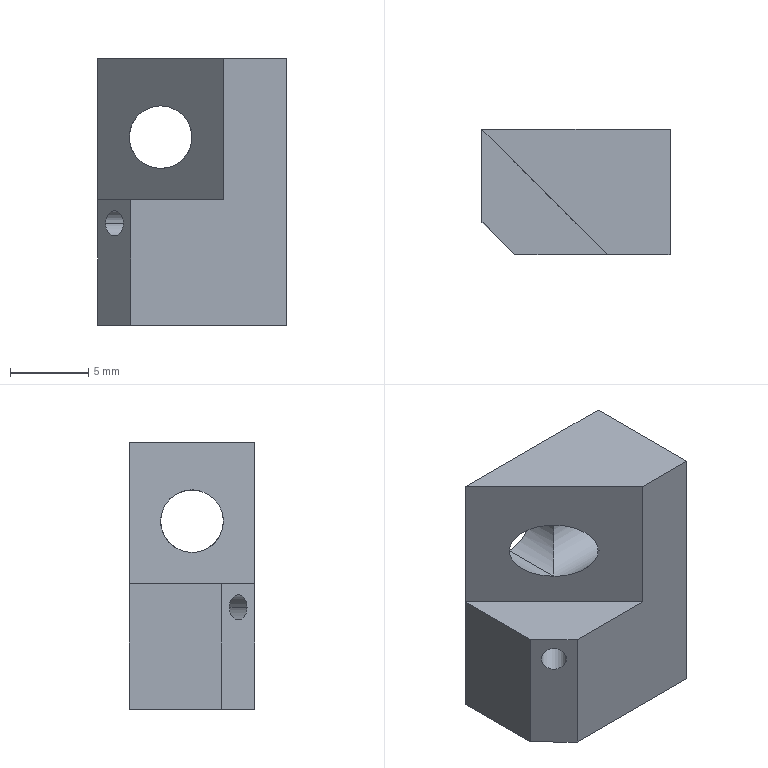NC program | NX | posted with a generic post | part box 12 x 8 x 17 mm
Whole program:
N10 G17 G21 G94 G90
(FLOOR_WALL , TOOL : D10JING)
N12 T09 M6
N14 G54
N16 G17 G0 G90 X-16. Y4.997 S9500 M3
N18 G43 Z30. H9
N20 Z3.
N22 G94 G1 Z0. F1250.
N24 X-13.
N26 X13.
N28 Y1.999
N30 X-13.
N32 Y-1.
N34 X13.
N36 X16.
N38 Z3.
N40 G0 Z30.
N42 M5
(FLOOR_WALL_1 , TOOL : D6)
N44 T06 M6
N46 G54
N48 G17 G0 G90 X-0.777 Y-9. S9500 M3
N50 G43 Z30. H6
N52 Z-0.297
N54 G94 G1 X-1.759 Y-7.3 F1000.
N56 G3 X-2.278 Y-7. R0.6
N58 G1 X-5.143 F2500.
N60 X-9. Y-3.143
N62 Y2.586
N64 X-8.97
N66 X0.586 Y-6.97
N68 Y-7.
N70 X-2.278
N72 G3 X-2.798 Y-7.3 R0.6
N74 G1 X-3.779 Y-9.
N76 G0 X-0.777 Z-0.593
N78 G1 X-1.759 Y-7.3 F1000.
N80 G3 X-2.278 Y-7. R0.6
N82 G1 X-5.143 F2500.
N84 X-9. Y-3.143
N86 Y2.586
N88 X-8.97
N90 X0.586 Y-6.97
N92 Y-7.
N94 X-2.278
N96 G3 X-2.798 Y-7.3 R0.6
N98 G1 X-3.779 Y-9.
N100 G0 X-0.777 Z-0.89
N102 G1 X-1.759 Y-7.3 F1000.
N104 G3 X-2.278 Y-7. R0.6
N106 G1 X-5.143 F2500.
N108 X-9. Y-3.143
N110 Y2.586
N112 X-8.97
N114 X0.586 Y-6.97
N116 Y-7.
N118 X-2.278
N120 G3 X-2.798 Y-7.3 R0.6
N122 G1 X-3.779 Y-9.
N124 G0 X-0.777 Z-1.187
N126 G1 X-1.759 Y-7.3 F1000.
N128 G3 X-2.278 Y-7. R0.6
N130 G1 X-5.143 F2500.
N132 X-9. Y-3.143
N134 Y2.586
N136 X-8.97
N138 X0.586 Y-6.97
N140 Y-7.
N142 X-2.278
N144 G3 X-2.798 Y-7.3 R0.6
N146 G1 X-3.779 Y-9.
N148 G0 X-0.777 Z-1.483
N150 G1 X-1.759 Y-7.3 F1000.
N152 G3 X-2.278 Y-7. R0.6
N154 G1 X-5.143 F2500.
N156 X-9. Y-3.143
N158 Y2.586
N160 X-8.97
N162 X0.586 Y-6.97
N164 Y-7.
N166 X-2.278
N168 G3 X-2.798 Y-7.3 R0.6
N170 G1 X-3.779 Y-9.
N172 G0 X-0.777 Z-1.78
N174 G1 X-1.759 Y-7.3 F1000.
N176 G3 X-2.278 Y-7. R0.6
N178 G1 X-5.143 F2500.
N180 X-9. Y-3.143
N182 Y2.586
N184 X-8.97
N186 X0.586 Y-6.97
N188 Y-7.
N190 X-2.278
N192 G3 X-2.798 Y-7.3 R0.6
N194 G1 X-3.779 Y-9.
N196 G0 X-0.777 Z-2.077
N198 G1 X-1.759 Y-7.3 F1000.
N200 G3 X-2.278 Y-7. R0.6
N202 G1 X-5.143 F2500.
N204 X-9. Y-3.143
N206 Y2.586
N208 X-8.97
N210 X0.586 Y-6.97
N212 Y-7.
N214 X-2.278
N216 G3 X-2.798 Y-7.3 R0.6
N218 G1 X-3.779 Y-9.
N220 G0 X-0.777 Z-2.373
N222 G1 X-1.759 Y-7.3 F1000.
N224 G3 X-2.278 Y-7. R0.6
N226 G1 X-5.143 F2500.
N228 X-9. Y-3.143
N230 Y2.586
N232 X-8.97
N234 X0.586 Y-6.97
N236 Y-7.
N238 X-2.278
N240 G3 X-2.798 Y-7.3 R0.6
N242 G1 X-3.779 Y-9.
N244 G0 X-0.777 Z-2.67
N246 G1 X-1.759 Y-7.3 F1000.
N248 G3 X-2.278 Y-7. R0.6
N250 G1 X-5.143 F2500.
N252 X-9. Y-3.143
N254 Y2.586
N256 X-8.97
N258 X0.586 Y-6.97
N260 Y-7.
N262 X-2.278
N264 G3 X-2.798 Y-7.3 R0.6
N266 G1 X-3.779 Y-9.
N268 G0 X-0.777 Z-2.967
N270 G1 X-1.759 Y-7.3 F1000.
N272 G3 X-2.278 Y-7. R0.6
N274 G1 X-5.143 F2500.
N276 X-9. Y-3.143
N278 Y2.586
N280 X-8.97
N282 X0.586 Y-6.97
N284 Y-7.
N286 X-2.278
N288 G3 X-2.798 Y-7.3 R0.6
N290 G1 X-3.779 Y-9.
N292 G0 X-0.777 Z-3.263
N294 G1 X-1.759 Y-7.3 F1000.
N296 G3 X-2.278 Y-7. R0.6
N298 G1 X-5.143 F2500.
N300 X-9. Y-3.143
N302 Y2.586
N304 X-8.97
N306 X0.586 Y-6.97
N308 Y-7.
N310 X-2.278
N312 G3 X-2.798 Y-7.3 R0.6
N314 G1 X-3.779 Y-9.
N316 G0 X-0.777 Z-3.56
N318 G1 X-1.759 Y-7.3 F1000.
N320 G3 X-2.278 Y-7. R0.6
N322 G1 X-5.143 F2500.
N324 X-9. Y-3.143
N326 Y2.586
N328 X-8.97
N330 X0.586 Y-6.97
N332 Y-7.
N334 X-2.278
N336 G3 X-2.798 Y-7.3 R0.6
N338 G1 X-3.779 Y-9.
N340 G0 X-0.777 Z-3.857
N342 G1 X-1.759 Y-7.3 F1000.
N344 G3 X-2.278 Y-7. R0.6
N346 G1 X-5.143 F2500.
N348 X-9. Y-3.143
N350 Y2.586
N352 X-8.97
N354 X0.586 Y-6.97
N356 Y-7.
N358 X-2.278
N360 G3 X-2.798 Y-7.3 R0.6
N362 G1 X-3.779 Y-9.
N364 G0 X-0.777 Z-4.153
N366 G1 X-1.759 Y-7.3 F1000.
N368 G3 X-2.278 Y-7. R0.6
N370 G1 X-5.143 F2500.
N372 X-9. Y-3.143
N374 Y2.586
N376 X-8.97
N378 X0.586 Y-6.97
N380 Y-7.
N382 X-2.278
N384 G3 X-2.798 Y-7.3 R0.6
N386 G1 X-3.779 Y-9.
N388 G0 X-0.777 Z-4.45
N390 G1 X-1.759 Y-7.3 F1000.
N392 G3 X-2.278 Y-7. R0.6
N394 G1 X-5.143 F2500.
N396 X-9. Y-3.143
N398 Y2.586
N400 X-8.97
N402 X0.586 Y-6.97
N404 Y-7.
N406 X-2.278
N408 G3 X-2.798 Y-7.3 R0.6
N410 G1 X-3.779 Y-9.
N412 G0 X-0.777 Z-4.747
N414 G1 X-1.759 Y-7.3 F1000.
N416 G3 X-2.278 Y-7. R0.6
N418 G1 X-5.143 F2500.
N420 X-9. Y-3.143
N422 Y2.586
N424 X-8.97
N426 X0.586 Y-6.97
N428 Y-7.
N430 X-2.278
N432 G3 X-2.798 Y-7.3 R0.6
N434 G1 X-3.779 Y-9.
N436 G0 X-0.777 Z-5.043
N438 G1 X-1.759 Y-7.3 F1000.
N440 G3 X-2.278 Y-7. R0.6
N442 G1 X-5.143 F2500.
N444 X-9. Y-3.143
N446 Y2.586
N448 X-8.97
N450 X0.586 Y-6.97
N452 Y-7.
N454 X-2.278
N456 G3 X-2.798 Y-7.3 R0.6
N458 G1 X-3.779 Y-9.
N460 G0 X-0.777 Z-5.34
N462 G1 X-1.759 Y-7.3 F1000.
N464 G3 X-2.278 Y-7. R0.6
N466 G1 X-5.143 F2500.
N468 X-9. Y-3.143
N470 Y2.586
N472 X-8.97
N474 X0.586 Y-6.97
N476 Y-7.
N478 X-2.278
N480 G3 X-2.798 Y-7.3 R0.6
N482 G1 X-3.779 Y-9.
N484 G0 X-0.777 Z-5.637
N486 G1 X-1.759 Y-7.3 F1000.
N488 G3 X-2.278 Y-7. R0.6
N490 G1 X-5.143 F2500.
N492 X-9. Y-3.143
N494 Y2.586
N496 X-8.97
N498 X0.586 Y-6.97
N500 Y-7.
N502 X-2.278
N504 G3 X-2.798 Y-7.3 R0.6
N506 G1 X-3.779 Y-9.
N508 G0 X-0.777 Z-5.933
N510 G1 X-1.759 Y-7.3 F1000.
N512 G3 X-2.278 Y-7. R0.6
N514 G1 X-5.143 F2500.
N516 X-9. Y-3.143
N518 Y2.586
N520 X-8.97
N522 X0.586 Y-6.97
N524 Y-7.
N526 X-2.278
N528 G3 X-2.798 Y-7.3 R0.6
N530 G1 X-3.779 Y-9.
N532 G0 X-0.777 Z-6.23
N534 G1 X-1.759 Y-7.3 F1000.
N536 G3 X-2.278 Y-7. R0.6
N538 G1 X-5.143 F2500.
N540 X-9. Y-3.143
N542 Y2.586
N544 X-8.97
N546 X0.586 Y-6.97
N548 Y-7.
N550 X-2.278
N552 G3 X-2.798 Y-7.3 R0.6
N554 G1 X-3.779 Y-9.
N556 G0 X-0.777 Z-6.527
N558 G1 X-1.759 Y-7.3 F1000.
N560 G3 X-2.278 Y-7. R0.6
N562 G1 X-5.143 F2500.
N564 X-9. Y-3.143
N566 Y2.586
N568 X-8.97
N570 X0.586 Y-6.97
N572 Y-7.
N574 X-2.278
N576 G3 X-2.798 Y-7.3 R0.6
N578 G1 X-3.779 Y-9.
N580 G0 X-0.777 Z-6.823
N582 G1 X-1.759 Y-7.3 F1000.
N584 G3 X-2.278 Y-7. R0.6
N586 G1 X-5.143 F2500.
N588 X-9. Y-3.143
N590 Y2.586
N592 X-8.97
N594 X0.586 Y-6.97
N596 Y-7.
N598 X-2.278
N600 G3 X-2.798 Y-7.3 R0.6
N602 G1 X-3.779 Y-9.
N604 G0 X-0.777 Z-7.12
N606 G1 X-1.759 Y-7.3 F1000.
N608 G3 X-2.278 Y-7. R0.6
N610 G1 X-5.143 F2500.
N612 X-9. Y-3.143
N614 Y2.586
N616 X-8.97
N618 X0.586 Y-6.97
N620 Y-7.
N622 X-2.278
N624 G3 X-2.798 Y-7.3 R0.6
N626 G1 X-3.779 Y-9.
N628 G0 X-0.777 Z-7.417
N630 G1 X-1.759 Y-7.3 F1000.
N632 G3 X-2.278 Y-7. R0.6
N634 G1 X-5.143 F2500.
N636 X-9. Y-3.143
N638 Y2.586
N640 X-8.97
N642 X0.586 Y-6.97
N644 Y-7.
N646 X-2.278
N648 G3 X-2.798 Y-7.3 R0.6
N650 G1 X-3.779 Y-9.
N652 G0 X-0.777 Z-7.713
N654 G1 X-1.759 Y-7.3 F1000.
N656 G3 X-2.278 Y-7. R0.6
N658 G1 X-5.143 F2500.
N660 X-9. Y-3.143
N662 Y2.586
N664 X-8.97
N666 X0.586 Y-6.97
N668 Y-7.
N670 X-2.278
N672 G3 X-2.798 Y-7.3 R0.6
N674 G1 X-3.779 Y-9.
N676 G0 X-0.777 Z-8.01
N678 G1 X-1.759 Y-7.3 F1000.
N680 G3 X-2.278 Y-7. R0.6
N682 G1 X-5.143 F2500.
N684 X-9. Y-3.143
N686 Y2.586
N688 X-8.97
N690 X0.586 Y-6.97
N692 Y-7.
N694 X-2.278
N696 G3 X-2.798 Y-7.3 R0.6
N698 G1 X-3.779 Y-9.
N700 G0 X-0.777 Z-8.307
N702 G1 X-1.759 Y-7.3 F1000.
N704 G3 X-2.278 Y-7. R0.6
N706 G1 X-5.143 F2500.
N708 X-9. Y-3.143
N710 Y2.586
N712 X-8.97
N714 X0.586 Y-6.97
N716 Y-7.
N718 X-2.278
N720 G3 X-2.798 Y-7.3 R0.6
N722 G1 X-3.779 Y-9.
N724 G0 X-0.777 Z-8.603
N726 G1 X-1.759 Y-7.3 F1000.
N728 G3 X-2.278 Y-7. R0.6
N730 G1 X-5.143 F2500.
N732 X-9. Y-3.143
N734 Y2.586
N736 X-8.97
N738 X0.586 Y-6.97
N740 Y-7.
N742 X-2.278
N744 G3 X-2.798 Y-7.3 R0.6
N746 G1 X-3.779 Y-9.
N748 G0 X-0.777 Z-8.9
N750 G1 X-1.759 Y-7.3 F1000.
N752 G3 X-2.278 Y-7. R0.6
N754 G1 X-5.143 F2500.
N756 X-9. Y-3.143
N758 Y2.586
N760 X-8.97
N762 X0.586 Y-6.97
N764 Y-7.
N766 X-2.278
N768 G3 X-2.798 Y-7.3 R0.6
N770 G1 X-3.779 Y-9.
N772 G0 Z30.
(FLOOR_WALL_1_COPY , TOOL : D6)
N774 X-0.904
N776 Z-9.
N778 G1 X-1.885 Y-7.3 F1000.
N780 G3 X-2.405 Y-7. R0.6
N782 G1 X-5.143 F1200.
N784 X-9. Y-3.143
N786 Y2.333
N788 X0.333 Y-7.
N790 X-2.405
N792 G3 X-2.924 Y-7.3 R0.6
N794 G1 X-3.906 Y-9.
N796 X0.532
N798 X0.913 Y-7.58 F1000.
N800 G3 X0.757 Y-7. R0.6
N802 G1 X-9. Y2.757 F1200.
N804 G3 X-9.58 Y2.913 R0.6
N806 G1 X-11.476 Y2.405
N808 G0 Z30.
N810 M5
(ZLEVEL_PROFILE_1_COPY , TOOL : D6A45)
N812 T07 M6
N814 G54
N816 G17 G0 G90 X-6.923 Y5.953 S9500 M3
N818 G43 Z30. H7
N820 Z1.
N822 G94 G1 Z-1. F1250.
N824 X-6.522 Y5.259
N826 G3 X-6.003 Y4.959 R0.6
N828 G1 X6.003
N830 G2 X6.959 Y4.003 R0.956
N832 G1 Y-4.003
N834 G2 X6.003 Y-4.959 R0.956
N836 G1 X1.997
N838 G2 X1.324 Y-4.68 R0.952
N840 G1 X-6.68 Y3.324
N842 G2 X-6.003 Y4.959 R0.957
N844 G3 X-5.483 Y5.259 R0.6
N846 G1 X-4.963 Y6.159
N848 Z1.
N850 G0 Z30.
N852 M5
(ZLEVEL_PROFILE_COPY_COPY_COPY_COPY_COPY , TOOL : D6)
N854 T06 M6
N856 G54
N858 G17 G0 G90 X-6.973 Y8.086 S9500 M3
N860 G43 Z30. H6
N862 Z-8.5
N864 G94 G1 Z-10. F1000.
N866 X-6.52 Y7.3
N868 G3 X-6. Y7. R0.6
N870 G1 X6. F1200.
N872 G2 X9. Y4. R3.
N874 G1 Y-4.
N876 G2 X6. Y-7. R3.
N878 G1 X-3.9
N880 G2 X-6.021 Y-6.121 R3.
N882 G1 X-8.121 Y-4.021
N884 G2 X-9. Y-1.9 R3.
N886 G1 Y4.
N888 G2 X-6. Y7. R3.
N890 G1 X5.754 Z-11.863
N892 X5.927 Z-11.891
N894 X6.1 Y6.998 Z-11.918
N896 X6.273 Y6.988 Z-11.945
N898 X6.444 Y6.967 Z-11.973
N900 X6.614 Y6.936 Z-12.
N902 X6.782 Y6.896 Z-12.028
N904 X6.948 Y6.846 Z-12.055
N906 X7.11 Y6.787 Z-12.082
N908 X7.269 Y6.718 Z-12.11
N910 X7.423 Y6.641 Z-12.137
N912 X7.573 Y6.555 Z-12.165
N914 X7.718 Y6.46 Z-12.192
N916 X7.856 Y6.357 Z-12.219
N918 X7.989 Y6.246 Z-12.247
N920 X8.115 Y6.128 Z-12.274
N922 X8.234 Y6.002 Z-12.302
N924 X8.346 Y5.87 Z-12.329
N926 X8.449 Y5.732 Z-12.356
N928 X8.545 Y5.588 Z-12.384
N930 X8.632 Y5.439 Z-12.411
N932 X8.711 Y5.285 Z-12.439
N934 X8.78 Y5.127 Z-12.466
N936 X8.841 Y4.965 Z-12.493
N938 X8.891 Y4.8 Z-12.521
N940 X8.933 Y4.632 Z-12.548
N942 X8.964 Y4.462 Z-12.576
N944 X8.986 Y4.29 Z-12.603
N946 X8.998 Y4.118 Z-12.63
N948 X9. Y3.945 Z-12.658
N950 Y3.772 Z-12.685
N952 Y-3.833 Z-13.891
N954 Y-4.006 Z-13.918
N956 X8.995 Y-4.179 Z-13.946
N958 X8.979 Y-4.351 Z-13.973
N960 X8.954 Y-4.522 Z-14.
N962 X8.919 Y-4.691 Z-14.028
N964 X8.875 Y-4.858 Z-14.055
N966 X8.82 Y-5.023 Z-14.083
N968 X8.757 Y-5.183 Z-14.11
N970 X8.684 Y-5.34 Z-14.137
N972 X8.602 Y-5.492 Z-14.165
N974 X8.512 Y-5.64 Z-14.192
N976 X8.414 Y-5.782 Z-14.22
N978 X8.307 Y-5.918 Z-14.247
N980 X8.193 Y-6.047 Z-14.274
N982 X8.071 Y-6.17 Z-14.302
N984 X7.943 Y-6.286 Z-14.329
N986 X7.808 Y-6.394 Z-14.357
N988 X7.667 Y-6.494 Z-14.384
N990 X7.521 Y-6.586 Z-14.411
N992 X7.369 Y-6.669 Z-14.439
N994 X7.213 Y-6.744 Z-14.466
N996 X7.053 Y-6.809 Z-14.494
N998 X6.89 Y-6.865 Z-14.521
N1000 X6.723 Y-6.912 Z-14.548
N1002 X6.554 Y-6.948 Z-14.576
N1004 X6.384 Y-6.975 Z-14.603
N1006 X6.212 Y-6.993 Z-14.631
N1008 X6.039 Y-7. Z-14.658
N1010 X5.866 Z-14.685
N1012 X5.693 Z-14.713
N1014 X-3.641 Z-16.192
N1016 X-3.814 Z-16.22
N1018 X-3.987 Y-6.999 Z-16.247
N1020 X-4.159 Y-6.989 Z-16.275
N1022 X-4.331 Y-6.969 Z-16.302
N1024 X-4.501 Y-6.939 Z-16.329
N1026 X-4.67 Y-6.9 Z-16.357
N1028 X-4.835 Y-6.85 Z-16.384
N1030 X-4.998 Y-6.792 Z-16.412
N1032 X-5.157 Y-6.724 Z-16.439
N1034 X-5.312 Y-6.647 Z-16.466
N1036 X-5.462 Y-6.561 Z-16.494
N1038 X-5.607 Y-6.467 Z-16.521
N1040 X-5.746 Y-6.365 Z-16.549
N1042 X-5.879 Y-6.255 Z-16.576
N1044 X-6.006 Y-6.137 Z-16.603
N1046 X-6.128 Y-6.015 Z-16.631
N1048 X-7.106 Y-5.037 Z-16.85
N1050 X-8.121 Y-4.021
N1052 G2 X-9. Y-1.9 R3.
N1054 G1 Y4.
N1056 G2 X-6. Y7. R3.
N1058 G1 X6.
N1060 G2 X9. Y4. R3.
N1062 G1 Y-4.
N1064 G2 X6. Y-7. R3.
N1066 G1 X-3.9
N1068 G2 X-6.021 Y-6.121 R3.
N1070 G1 X-7.106 Y-5.037
N1072 G3 X-7.685 Y-4.882 R0.6
N1074 G1 X-8.689 Y-5.151
N1076 Z-15.35
N1078 G0 Z30.
N1080 M5
N1082 M2